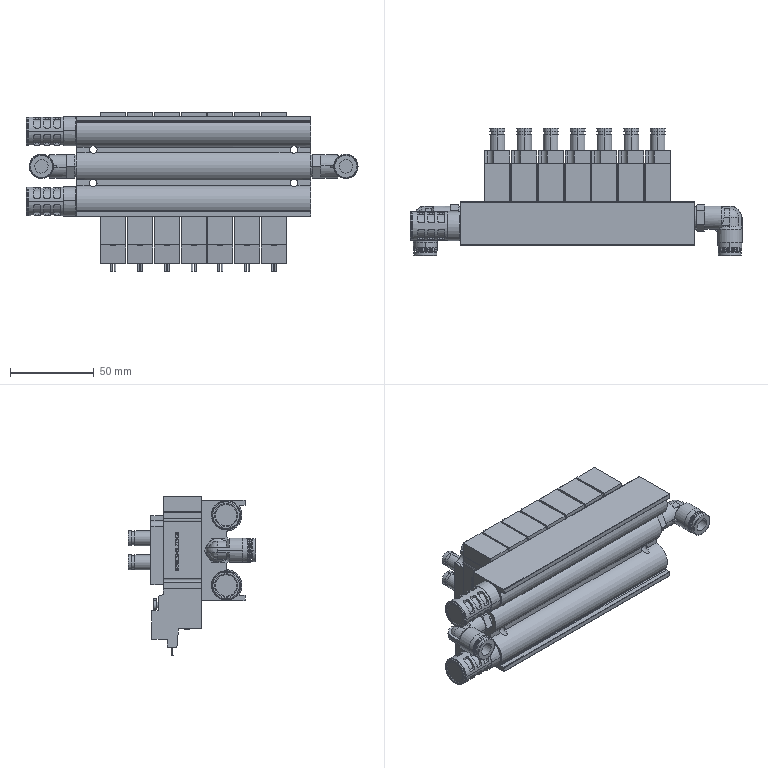Part | NX | 12 solids | 4892 faces | volume 410655 mm3 | plane 4170 | cylinder 576 | cone 132 | torus 8 | sphere 4 | spline 2 | commonest cylinder face diameters 2 x96 4 x84 9 x56 2.5 x42 7.938 x42 14 x36